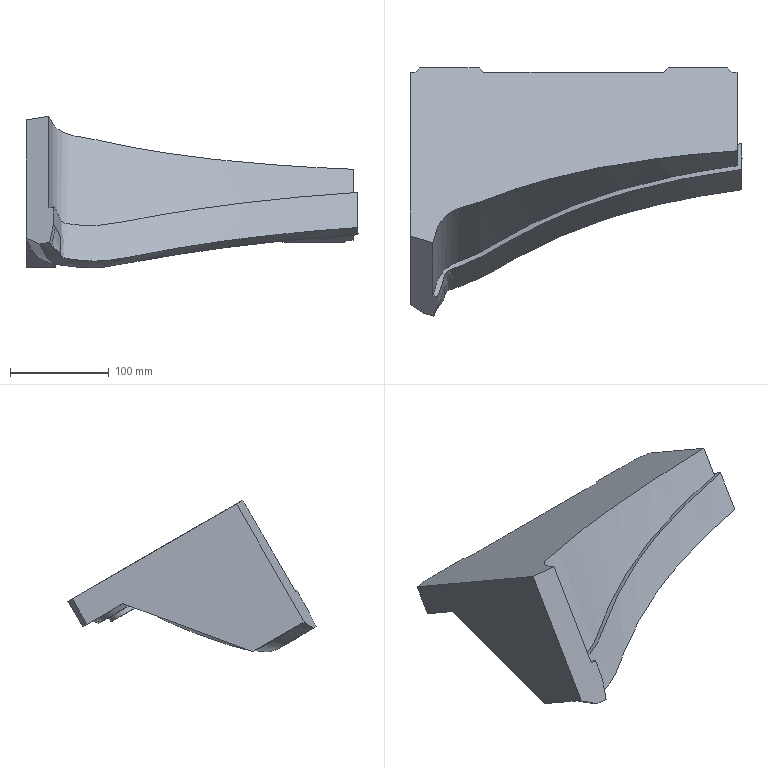Part | NX | features solid 2 | 1 solid | 41 faces | box 336.667 x 251.534 x 153.956 mm | volume 2324857 mm3 | plane 24 | spline 11 | cone 4 | cylinder 2 | commonest cylinder face diameters 30 x2